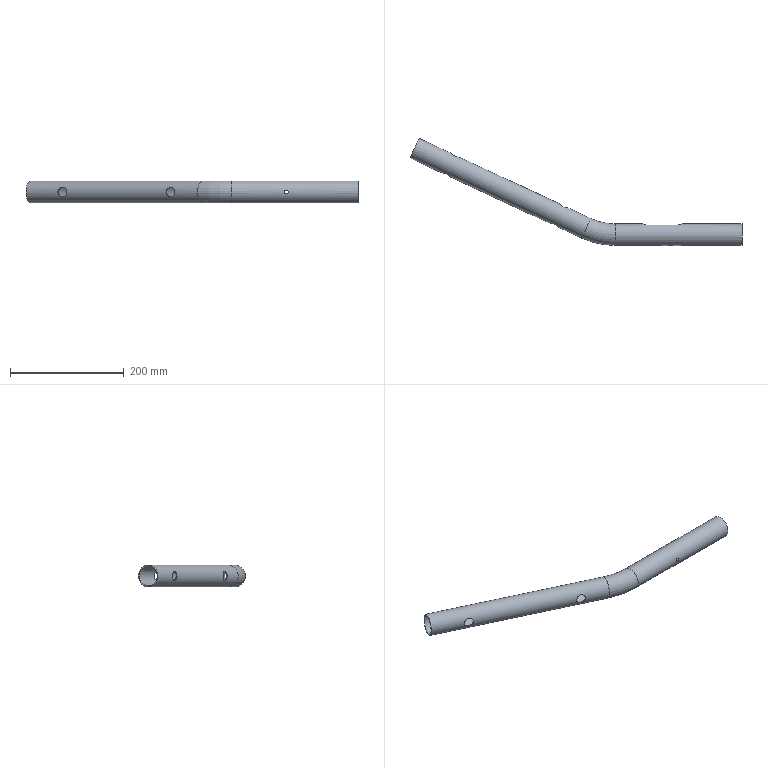Part | STEP file | 6151201L | 1 solid | 17 faces | box 584.322 x 188.458 x 38.1 mm | volume 101738 mm3 | cylinder 11 | plane 4 | torus 2 | commonest cylinder face diameters 17 x4 18 x2 35.1 x2 38.1 x2 7 x1